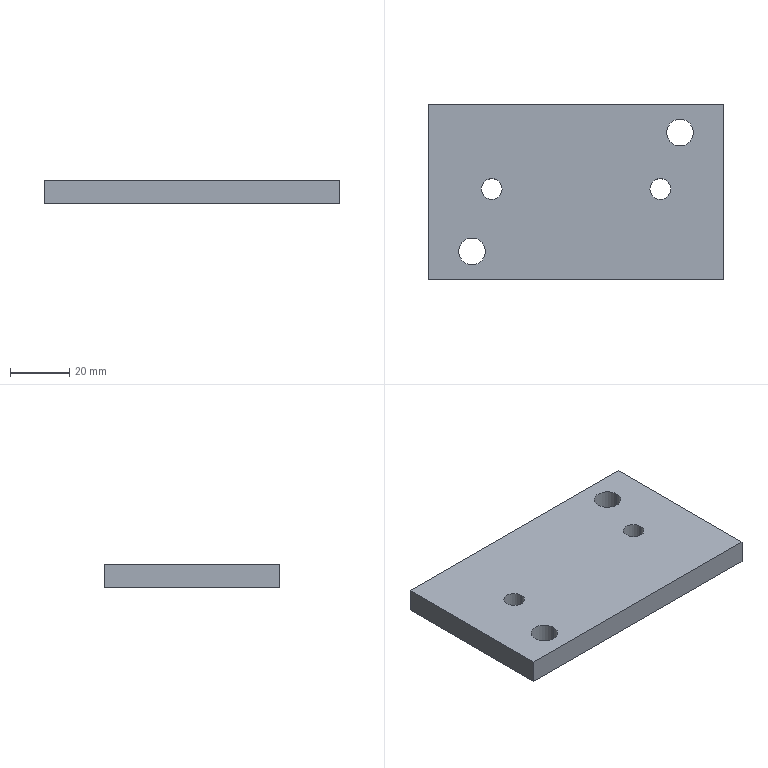Part | 1 solid | 14 faces | box 99 x 59 x 8 mm | volume 45095 mm3 | cylinder 8 | plane 6 | commonest cylinder face diameters 7 x4 9 x4
STEP:
#1=CARTESIAN_POINT('',(0.,0.,0.));
#2=DIRECTION('',(0.,0.,1.));
#3=DIRECTION('',(1.,0.,0.));
#4=AXIS2_PLACEMENT_3D('',#1,#2,#3);
#5=CARTESIAN_POINT('',(-190.5,445.,-105.051));
#6=VERTEX_POINT('',#5);
#7=CARTESIAN_POINT('',(-190.5,504.,-105.051));
#8=VERTEX_POINT('',#7);
#9=CARTESIAN_POINT('',(-190.5,445.,-105.051));
#10=DIRECTION('',(0.,1.,0.));
#11=VECTOR('',#10,1.);
#12=LINE('',#9,#11);
#13=CARTESIAN_POINT('',(-190.5,445.,-113.051));
#14=DIRECTION('',(1.,0.,0.));
#15=DIRECTION('',(0.,0.,1.));
#16=AXIS2_PLACEMENT_3D('',#13,#14,#15);
#17=PLANE('',#16);
#18=CARTESIAN_POINT('',(8.,0.));
#19=DIRECTION('',(0.,-1.));
#20=VECTOR('',#19,1.);
#21=LINE('',#18,#20);
#22=(GEOMETRIC_REPRESENTATION_CONTEXT(2)PARAMETRIC_REPRESENTATION_CONTEXT()REPRESENTATION_CONTEXT('',''));
#23=DEFINITIONAL_REPRESENTATION('',(#21),#22);
#24=PCURVE('',#17,#23);
#25=CARTESIAN_POINT('',(-211.613,475.5,-105.051));
#26=DIRECTION('',(0.,0.,1.));
#27=DIRECTION('',(-1.,0.,0.));
#28=AXIS2_PLACEMENT_3D('',#25,#26,#27);
#29=PLANE('',#28);
#30=CARTESIAN_POINT('',(-21.113,30.5));
#31=DIRECTION('',(0.,-1.));
#32=VECTOR('',#31,1.);
#33=LINE('',#30,#32);
#34=(GEOMETRIC_REPRESENTATION_CONTEXT(2)PARAMETRIC_REPRESENTATION_CONTEXT()REPRESENTATION_CONTEXT('',''));
#35=DEFINITIONAL_REPRESENTATION('',(#33),#34);
#36=PCURVE('',#29,#35);
#37=SURFACE_CURVE('',#12,(#24,#36),.PCURVE_S1.);
#38=EDGE_CURVE('',#6,#8,#37,.T.);
#39=ORIENTED_EDGE('',*,*,#38,.F.);
#40=CARTESIAN_POINT('',(-190.5,445.,-113.051));
#41=VERTEX_POINT('',#40);
#42=CARTESIAN_POINT('',(-190.5,445.,-113.051));
#43=DIRECTION('',(0.,0.,1.));
#44=VECTOR('',#43,1.);
#45=LINE('',#42,#44);
#46=CARTESIAN_POINT('',(0.,0.));
#47=DIRECTION('',(1.,0.));
#48=VECTOR('',#47,1.);
#49=LINE('',#46,#48);
#50=(GEOMETRIC_REPRESENTATION_CONTEXT(2)PARAMETRIC_REPRESENTATION_CONTEXT()REPRESENTATION_CONTEXT('',''));
#51=DEFINITIONAL_REPRESENTATION('',(#49),#50);
#52=PCURVE('',#17,#51);
#53=CARTESIAN_POINT('',(-289.5,445.,-113.051));
#54=DIRECTION('',(0.,-1.,0.));
#55=DIRECTION('',(0.,0.,1.));
#56=AXIS2_PLACEMENT_3D('',#53,#54,#55);
#57=PLANE('',#56);
#58=CARTESIAN_POINT('',(0.,-99.));
#59=DIRECTION('',(1.,0.));
#60=VECTOR('',#59,1.);
#61=LINE('',#58,#60);
#62=(GEOMETRIC_REPRESENTATION_CONTEXT(2)PARAMETRIC_REPRESENTATION_CONTEXT()REPRESENTATION_CONTEXT('',''));
#63=DEFINITIONAL_REPRESENTATION('',(#61),#62);
#64=PCURVE('',#57,#63);
#65=SURFACE_CURVE('',#45,(#52,#64),.PCURVE_S1.);
#66=EDGE_CURVE('',#41,#6,#65,.T.);
#67=ORIENTED_EDGE('',*,*,#66,.F.);
#68=CARTESIAN_POINT('',(-190.5,504.,-113.051));
#69=VERTEX_POINT('',#68);
#70=CARTESIAN_POINT('',(-190.5,445.,-113.051));
#71=DIRECTION('',(0.,1.,0.));
#72=VECTOR('',#71,1.);
#73=LINE('',#70,#72);
#74=CARTESIAN_POINT('',(0.,0.));
#75=DIRECTION('',(0.,-1.));
#76=VECTOR('',#75,1.);
#77=LINE('',#74,#76);
#78=(GEOMETRIC_REPRESENTATION_CONTEXT(2)PARAMETRIC_REPRESENTATION_CONTEXT()REPRESENTATION_CONTEXT('',''));
#79=DEFINITIONAL_REPRESENTATION('',(#77),#78);
#80=PCURVE('',#17,#79);
#81=CARTESIAN_POINT('',(-211.613,475.5,-113.051));
#82=DIRECTION('',(0.,0.,1.));
#83=DIRECTION('',(-1.,0.,0.));
#84=AXIS2_PLACEMENT_3D('',#81,#82,#83);
#85=PLANE('',#84);
#86=CARTESIAN_POINT('',(-21.113,30.5));
#87=DIRECTION('',(0.,-1.));
#88=VECTOR('',#87,1.);
#89=LINE('',#86,#88);
#90=(GEOMETRIC_REPRESENTATION_CONTEXT(2)PARAMETRIC_REPRESENTATION_CONTEXT()REPRESENTATION_CONTEXT('',''));
#91=DEFINITIONAL_REPRESENTATION('',(#89),#90);
#92=PCURVE('',#85,#91);
#93=SURFACE_CURVE('',#73,(#80,#92),.PCURVE_S1.);
#94=EDGE_CURVE('',#41,#69,#93,.T.);
#95=ORIENTED_EDGE('',*,*,#94,.T.);
#96=CARTESIAN_POINT('',(-190.5,504.,-113.051));
#97=DIRECTION('',(0.,0.,1.));
#98=VECTOR('',#97,1.);
#99=LINE('',#96,#98);
#100=CARTESIAN_POINT('',(0.,-59.));
#101=DIRECTION('',(1.,0.));
#102=VECTOR('',#101,1.);
#103=LINE('',#100,#102);
#104=(GEOMETRIC_REPRESENTATION_CONTEXT(2)PARAMETRIC_REPRESENTATION_CONTEXT()REPRESENTATION_CONTEXT('',''));
#105=DEFINITIONAL_REPRESENTATION('',(#103),#104);
#106=PCURVE('',#17,#105);
#107=CARTESIAN_POINT('',(-190.5,504.,-113.051));
#108=DIRECTION('',(0.,1.,0.));
#109=DIRECTION('',(0.,0.,-1.));
#110=AXIS2_PLACEMENT_3D('',#107,#108,#109);
#111=PLANE('',#110);
#112=CARTESIAN_POINT('',(0.,0.));
#113=DIRECTION('',(-1.,0.));
#114=VECTOR('',#113,1.);
#115=LINE('',#112,#114);
#116=(GEOMETRIC_REPRESENTATION_CONTEXT(2)PARAMETRIC_REPRESENTATION_CONTEXT()REPRESENTATION_CONTEXT('',''));
#117=DEFINITIONAL_REPRESENTATION('',(#115),#116);
#118=PCURVE('',#111,#117);
#119=SURFACE_CURVE('',#99,(#106,#118),.PCURVE_S1.);
#120=EDGE_CURVE('',#69,#8,#119,.T.);
#121=ORIENTED_EDGE('',*,*,#120,.T.);
#122=EDGE_LOOP('',(#39,#67,#95,#121));
#123=FACE_BOUND('',#122,.T.);
#124=ADVANCED_FACE('',(#123),#17,.T.);
#125=CARTESIAN_POINT('',(-289.5,504.,-105.051));
#126=VERTEX_POINT('',#125);
#127=CARTESIAN_POINT('',(-190.5,504.,-105.051));
#128=DIRECTION('',(-1.,0.,0.));
#129=VECTOR('',#128,1.);
#130=LINE('',#127,#129);
#131=CARTESIAN_POINT('',(-8.,0.));
#132=DIRECTION('',(0.,1.));
#133=VECTOR('',#132,1.);
#134=LINE('',#131,#133);
#135=(GEOMETRIC_REPRESENTATION_CONTEXT(2)PARAMETRIC_REPRESENTATION_CONTEXT()REPRESENTATION_CONTEXT('',''));
#136=DEFINITIONAL_REPRESENTATION('',(#134),#135);
#137=PCURVE('',#111,#136);
#138=CARTESIAN_POINT('',(-21.113,-28.5));
#139=DIRECTION('',(1.,0.));
#140=VECTOR('',#139,1.);
#141=LINE('',#138,#140);
#142=(GEOMETRIC_REPRESENTATION_CONTEXT(2)PARAMETRIC_REPRESENTATION_CONTEXT()REPRESENTATION_CONTEXT('',''));
#143=DEFINITIONAL_REPRESENTATION('',(#141),#142);
#144=PCURVE('',#29,#143);
#145=SURFACE_CURVE('',#130,(#137,#144),.PCURVE_S1.);
#146=EDGE_CURVE('',#8,#126,#145,.T.);
#147=ORIENTED_EDGE('',*,*,#146,.F.);
#148=ORIENTED_EDGE('',*,*,#120,.F.);
#149=CARTESIAN_POINT('',(-289.5,504.,-113.051));
#150=VERTEX_POINT('',#149);
#151=CARTESIAN_POINT('',(-190.5,504.,-113.051));
#152=DIRECTION('',(-1.,0.,0.));
#153=VECTOR('',#152,1.);
#154=LINE('',#151,#153);
#155=CARTESIAN_POINT('',(0.,0.));
#156=DIRECTION('',(0.,1.));
#157=VECTOR('',#156,1.);
#158=LINE('',#155,#157);
#159=(GEOMETRIC_REPRESENTATION_CONTEXT(2)PARAMETRIC_REPRESENTATION_CONTEXT()REPRESENTATION_CONTEXT('',''));
#160=DEFINITIONAL_REPRESENTATION('',(#158),#159);
#161=PCURVE('',#111,#160);
#162=CARTESIAN_POINT('',(-21.113,-28.5));
#163=DIRECTION('',(1.,0.));
#164=VECTOR('',#163,1.);
#165=LINE('',#162,#164);
#166=(GEOMETRIC_REPRESENTATION_CONTEXT(2)PARAMETRIC_REPRESENTATION_CONTEXT()REPRESENTATION_CONTEXT('',''));
#167=DEFINITIONAL_REPRESENTATION('',(#165),#166);
#168=PCURVE('',#85,#167);
#169=SURFACE_CURVE('',#154,(#161,#168),.PCURVE_S1.);
#170=EDGE_CURVE('',#69,#150,#169,.T.);
#171=ORIENTED_EDGE('',*,*,#170,.T.);
#172=CARTESIAN_POINT('',(-289.5,504.,-113.051));
#173=DIRECTION('',(0.,0.,1.));
#174=VECTOR('',#173,1.);
#175=LINE('',#172,#174);
#176=CARTESIAN_POINT('',(0.,99.));
#177=DIRECTION('',(-1.,0.));
#178=VECTOR('',#177,1.);
#179=LINE('',#176,#178);
#180=(GEOMETRIC_REPRESENTATION_CONTEXT(2)PARAMETRIC_REPRESENTATION_CONTEXT()REPRESENTATION_CONTEXT('',''));
#181=DEFINITIONAL_REPRESENTATION('',(#179),#180);
#182=PCURVE('',#111,#181);
#183=CARTESIAN_POINT('',(-289.5,504.,-113.051));
#184=DIRECTION('',(-1.,0.,0.));
#185=DIRECTION('',(0.,0.,-1.));
#186=AXIS2_PLACEMENT_3D('',#183,#184,#185);
#187=PLANE('',#186);
#188=CARTESIAN_POINT('',(0.,0.));
#189=DIRECTION('',(-1.,0.));
#190=VECTOR('',#189,1.);
#191=LINE('',#188,#190);
#192=(GEOMETRIC_REPRESENTATION_CONTEXT(2)PARAMETRIC_REPRESENTATION_CONTEXT()REPRESENTATION_CONTEXT('',''));
#193=DEFINITIONAL_REPRESENTATION('',(#191),#192);
#194=PCURVE('',#187,#193);
#195=SURFACE_CURVE('',#175,(#182,#194),.PCURVE_S1.);
#196=EDGE_CURVE('',#150,#126,#195,.T.);
#197=ORIENTED_EDGE('',*,*,#196,.T.);
#198=EDGE_LOOP('',(#147,#148,#171,#197));
#199=FACE_BOUND('',#198,.T.);
#200=ADVANCED_FACE('',(#199),#111,.T.);
#201=CARTESIAN_POINT('',(-289.5,445.,-105.051));
#202=VERTEX_POINT('',#201);
#203=CARTESIAN_POINT('',(-289.5,504.,-105.051));
#204=DIRECTION('',(0.,-1.,0.));
#205=VECTOR('',#204,1.);
#206=LINE('',#203,#205);
#207=CARTESIAN_POINT('',(-8.,0.));
#208=DIRECTION('',(0.,1.));
#209=VECTOR('',#208,1.);
#210=LINE('',#207,#209);
#211=(GEOMETRIC_REPRESENTATION_CONTEXT(2)PARAMETRIC_REPRESENTATION_CONTEXT()REPRESENTATION_CONTEXT('',''));
#212=DEFINITIONAL_REPRESENTATION('',(#210),#211);
#213=PCURVE('',#187,#212);
#214=CARTESIAN_POINT('',(77.887,-28.5));
#215=DIRECTION('',(0.,1.));
#216=VECTOR('',#215,1.);
#217=LINE('',#214,#216);
#218=(GEOMETRIC_REPRESENTATION_CONTEXT(2)PARAMETRIC_REPRESENTATION_CONTEXT()REPRESENTATION_CONTEXT('',''));
#219=DEFINITIONAL_REPRESENTATION('',(#217),#218);
#220=PCURVE('',#29,#219);
#221=SURFACE_CURVE('',#206,(#213,#220),.PCURVE_S1.);
#222=EDGE_CURVE('',#126,#202,#221,.T.);
#223=ORIENTED_EDGE('',*,*,#222,.F.);
#224=ORIENTED_EDGE('',*,*,#196,.F.);
#225=CARTESIAN_POINT('',(-289.5,445.,-113.051));
#226=VERTEX_POINT('',#225);
#227=CARTESIAN_POINT('',(-289.5,504.,-113.051));
#228=DIRECTION('',(0.,-1.,0.));
#229=VECTOR('',#228,1.);
#230=LINE('',#227,#229);
#231=CARTESIAN_POINT('',(0.,0.));
#232=DIRECTION('',(0.,1.));
#233=VECTOR('',#232,1.);
#234=LINE('',#231,#233);
#235=(GEOMETRIC_REPRESENTATION_CONTEXT(2)PARAMETRIC_REPRESENTATION_CONTEXT()REPRESENTATION_CONTEXT('',''));
#236=DEFINITIONAL_REPRESENTATION('',(#234),#235);
#237=PCURVE('',#187,#236);
#238=CARTESIAN_POINT('',(77.887,-28.5));
#239=DIRECTION('',(0.,1.));
#240=VECTOR('',#239,1.);
#241=LINE('',#238,#240);
#242=(GEOMETRIC_REPRESENTATION_CONTEXT(2)PARAMETRIC_REPRESENTATION_CONTEXT()REPRESENTATION_CONTEXT('',''));
#243=DEFINITIONAL_REPRESENTATION('',(#241),#242);
#244=PCURVE('',#85,#243);
#245=SURFACE_CURVE('',#230,(#237,#244),.PCURVE_S1.);
#246=EDGE_CURVE('',#150,#226,#245,.T.);
#247=ORIENTED_EDGE('',*,*,#246,.T.);
#248=CARTESIAN_POINT('',(-289.5,445.,-113.051));
#249=DIRECTION('',(0.,0.,1.));
#250=VECTOR('',#249,1.);
#251=LINE('',#248,#250);
#252=CARTESIAN_POINT('',(0.,59.));
#253=DIRECTION('',(-1.,0.));
#254=VECTOR('',#253,1.);
#255=LINE('',#252,#254);
#256=(GEOMETRIC_REPRESENTATION_CONTEXT(2)PARAMETRIC_REPRESENTATION_CONTEXT()REPRESENTATION_CONTEXT('',''));
#257=DEFINITIONAL_REPRESENTATION('',(#255),#256);
#258=PCURVE('',#187,#257);
#259=CARTESIAN_POINT('',(0.,0.));
#260=DIRECTION('',(1.,0.));
#261=VECTOR('',#260,1.);
#262=LINE('',#259,#261);
#263=(GEOMETRIC_REPRESENTATION_CONTEXT(2)PARAMETRIC_REPRESENTATION_CONTEXT()REPRESENTATION_CONTEXT('',''));
#264=DEFINITIONAL_REPRESENTATION('',(#262),#263);
#265=PCURVE('',#57,#264);
#266=SURFACE_CURVE('',#251,(#258,#265),.PCURVE_S1.);
#267=EDGE_CURVE('',#226,#202,#266,.T.);
#268=ORIENTED_EDGE('',*,*,#267,.T.);
#269=EDGE_LOOP('',(#223,#224,#247,#268));
#270=FACE_BOUND('',#269,.T.);
#271=ADVANCED_FACE('',(#270),#187,.T.);
#272=CARTESIAN_POINT('',(-289.5,445.,-105.051));
#273=DIRECTION('',(1.,0.,0.));
#274=VECTOR('',#273,1.);
#275=LINE('',#272,#274);
#276=CARTESIAN_POINT('',(8.,0.));
#277=DIRECTION('',(0.,-1.));
#278=VECTOR('',#277,1.);
#279=LINE('',#276,#278);
#280=(GEOMETRIC_REPRESENTATION_CONTEXT(2)PARAMETRIC_REPRESENTATION_CONTEXT()REPRESENTATION_CONTEXT('',''));
#281=DEFINITIONAL_REPRESENTATION('',(#279),#280);
#282=PCURVE('',#57,#281);
#283=CARTESIAN_POINT('',(77.887,30.5));
#284=DIRECTION('',(-1.,0.));
#285=VECTOR('',#284,1.);
#286=LINE('',#283,#285);
#287=(GEOMETRIC_REPRESENTATION_CONTEXT(2)PARAMETRIC_REPRESENTATION_CONTEXT()REPRESENTATION_CONTEXT('',''));
#288=DEFINITIONAL_REPRESENTATION('',(#286),#287);
#289=PCURVE('',#29,#288);
#290=SURFACE_CURVE('',#275,(#282,#289),.PCURVE_S1.);
#291=EDGE_CURVE('',#202,#6,#290,.T.);
#292=ORIENTED_EDGE('',*,*,#291,.F.);
#293=ORIENTED_EDGE('',*,*,#267,.F.);
#294=CARTESIAN_POINT('',(-289.5,445.,-113.051));
#295=DIRECTION('',(1.,0.,0.));
#296=VECTOR('',#295,1.);
#297=LINE('',#294,#296);
#298=CARTESIAN_POINT('',(0.,0.));
#299=DIRECTION('',(0.,-1.));
#300=VECTOR('',#299,1.);
#301=LINE('',#298,#300);
#302=(GEOMETRIC_REPRESENTATION_CONTEXT(2)PARAMETRIC_REPRESENTATION_CONTEXT()REPRESENTATION_CONTEXT('',''));
#303=DEFINITIONAL_REPRESENTATION('',(#301),#302);
#304=PCURVE('',#57,#303);
#305=CARTESIAN_POINT('',(77.887,30.5));
#306=DIRECTION('',(-1.,0.));
#307=VECTOR('',#306,1.);
#308=LINE('',#305,#307);
#309=(GEOMETRIC_REPRESENTATION_CONTEXT(2)PARAMETRIC_REPRESENTATION_CONTEXT()REPRESENTATION_CONTEXT('',''));
#310=DEFINITIONAL_REPRESENTATION('',(#308),#309);
#311=PCURVE('',#85,#310);
#312=SURFACE_CURVE('',#297,(#304,#311),.PCURVE_S1.);
#313=EDGE_CURVE('',#226,#41,#312,.T.);
#314=ORIENTED_EDGE('',*,*,#313,.T.);
#315=ORIENTED_EDGE('',*,*,#66,.T.);
#316=EDGE_LOOP('',(#292,#293,#314,#315));
#317=FACE_BOUND('',#316,.T.);
#318=ADVANCED_FACE('',(#317),#57,.T.);
#319=ORIENTED_EDGE('',*,*,#94,.F.);
#320=ORIENTED_EDGE('',*,*,#313,.F.);
#321=ORIENTED_EDGE('',*,*,#246,.F.);
#322=ORIENTED_EDGE('',*,*,#170,.F.);
#323=EDGE_LOOP('',(#319,#320,#321,#322));
#324=FACE_BOUND('',#323,.T.);
#325=CARTESIAN_POINT('',(-215.113,475.5,-113.051));
#326=VERTEX_POINT('',#325);
#327=CARTESIAN_POINT('',(-208.113,475.5,-113.051));
#328=VERTEX_POINT('',#327);
#329=CARTESIAN_POINT('',(-211.613,475.5,-113.051));
#330=DIRECTION('',(0.,0.,1.));
#331=DIRECTION('',(-1.,0.,0.));
#332=AXIS2_PLACEMENT_3D('',#329,#330,#331);
#333=CIRCLE('',#332,3.5);
#334=CARTESIAN_POINT('',(0.,0.));
#335=DIRECTION('',(1.,0.));
#336=AXIS2_PLACEMENT_2D('',#334,#335);
#337=CIRCLE('',#336,3.5);
#338=(GEOMETRIC_REPRESENTATION_CONTEXT(2)PARAMETRIC_REPRESENTATION_CONTEXT()REPRESENTATION_CONTEXT('',''));
#339=DEFINITIONAL_REPRESENTATION('',(#337),#338);
#340=PCURVE('',#85,#339);
#341=CARTESIAN_POINT('',(-211.613,475.5,-113.051));
#342=DIRECTION('',(0.,0.,1.));
#343=DIRECTION('',(0.,1.,0.));
#344=AXIS2_PLACEMENT_3D('',#341,#342,#343);
#345=CYLINDRICAL_SURFACE('',#344,3.5);
#346=CARTESIAN_POINT('',(1.571,0.));
#347=DIRECTION('',(1.,0.));
#348=VECTOR('',#347,1.);
#349=LINE('',#346,#348);
#350=(GEOMETRIC_REPRESENTATION_CONTEXT(2)PARAMETRIC_REPRESENTATION_CONTEXT()REPRESENTATION_CONTEXT('',''));
#351=DEFINITIONAL_REPRESENTATION('',(#349),#350);
#352=PCURVE('',#345,#351);
#353=SURFACE_CURVE('',#333,(#340,#352),.PCURVE_S1.);
#354=EDGE_CURVE('',#326,#328,#353,.T.);
#355=ORIENTED_EDGE('',*,*,#354,.T.);
#356=CARTESIAN_POINT('',(-211.613,475.5,-113.051));
#357=DIRECTION('',(0.,0.,1.));
#358=DIRECTION('',(-1.,0.,0.));
#359=AXIS2_PLACEMENT_3D('',#356,#357,#358);
#360=CIRCLE('',#359,3.5);
#361=CARTESIAN_POINT('',(0.,0.));
#362=DIRECTION('',(1.,0.));
#363=AXIS2_PLACEMENT_2D('',#361,#362);
#364=CIRCLE('',#363,3.5);
#365=(GEOMETRIC_REPRESENTATION_CONTEXT(2)PARAMETRIC_REPRESENTATION_CONTEXT()REPRESENTATION_CONTEXT('',''));
#366=DEFINITIONAL_REPRESENTATION('',(#364),#365);
#367=PCURVE('',#85,#366);
#368=CARTESIAN_POINT('',(-211.613,475.5,-113.051));
#369=DIRECTION('',(0.,0.,1.));
#370=DIRECTION('',(0.,-1.,0.));
#371=AXIS2_PLACEMENT_3D('',#368,#369,#370);
#372=CYLINDRICAL_SURFACE('',#371,3.5);
#373=CARTESIAN_POINT('',(-1.571,0.));
#374=DIRECTION('',(1.,0.));
#375=VECTOR('',#374,1.);
#376=LINE('',#373,#375);
#377=(GEOMETRIC_REPRESENTATION_CONTEXT(2)PARAMETRIC_REPRESENTATION_CONTEXT()REPRESENTATION_CONTEXT('',''));
#378=DEFINITIONAL_REPRESENTATION('',(#376),#377);
#379=PCURVE('',#372,#378);
#380=SURFACE_CURVE('',#360,(#367,#379),.PCURVE_S1.);
#381=EDGE_CURVE('',#328,#326,#380,.T.);
#382=ORIENTED_EDGE('',*,*,#381,.T.);
#383=EDGE_LOOP('',(#355,#382));
#384=FACE_BOUND('',#383,.T.);
#385=CARTESIAN_POINT('',(-209.5,494.5,-113.051));
#386=VERTEX_POINT('',#385);
#387=CARTESIAN_POINT('',(-200.5,494.5,-113.051));
#388=VERTEX_POINT('',#387);
#389=CARTESIAN_POINT('',(-205.,494.5,-113.051));
#390=DIRECTION('',(0.,0.,1.));
#391=DIRECTION('',(-1.,0.,0.));
#392=AXIS2_PLACEMENT_3D('',#389,#390,#391);
#393=CIRCLE('',#392,4.5);
#394=CARTESIAN_POINT('',(-6.613,-19.));
#395=DIRECTION('',(1.,0.));
#396=AXIS2_PLACEMENT_2D('',#394,#395);
#397=CIRCLE('',#396,4.5);
#398=(GEOMETRIC_REPRESENTATION_CONTEXT(2)PARAMETRIC_REPRESENTATION_CONTEXT()REPRESENTATION_CONTEXT('',''));
#399=DEFINITIONAL_REPRESENTATION('',(#397),#398);
#400=PCURVE('',#85,#399);
#401=CARTESIAN_POINT('',(-205.,494.5,-113.051));
#402=DIRECTION('',(0.,0.,1.));
#403=DIRECTION('',(0.,1.,0.));
#404=AXIS2_PLACEMENT_3D('',#401,#402,#403);
#405=CYLINDRICAL_SURFACE('',#404,4.5);
#406=CARTESIAN_POINT('',(1.571,0.));
#407=DIRECTION('',(1.,0.));
#408=VECTOR('',#407,1.);
#409=LINE('',#406,#408);
#410=(GEOMETRIC_REPRESENTATION_CONTEXT(2)PARAMETRIC_REPRESENTATION_CONTEXT()REPRESENTATION_CONTEXT('',''));
#411=DEFINITIONAL_REPRESENTATION('',(#409),#410);
#412=PCURVE('',#405,#411);
#413=SURFACE_CURVE('',#393,(#400,#412),.PCURVE_S1.);
#414=EDGE_CURVE('',#386,#388,#413,.T.);
#415=ORIENTED_EDGE('',*,*,#414,.T.);
#416=CARTESIAN_POINT('',(-205.,494.5,-113.051));
#417=DIRECTION('',(0.,0.,1.));
#418=DIRECTION('',(-1.,0.,0.));
#419=AXIS2_PLACEMENT_3D('',#416,#417,#418);
#420=CIRCLE('',#419,4.5);
#421=CARTESIAN_POINT('',(-6.613,-19.));
#422=DIRECTION('',(1.,0.));
#423=AXIS2_PLACEMENT_2D('',#421,#422);
#424=CIRCLE('',#423,4.5);
#425=(GEOMETRIC_REPRESENTATION_CONTEXT(2)PARAMETRIC_REPRESENTATION_CONTEXT()REPRESENTATION_CONTEXT('',''));
#426=DEFINITIONAL_REPRESENTATION('',(#424),#425);
#427=PCURVE('',#85,#426);
#428=CARTESIAN_POINT('',(-205.,494.5,-113.051));
#429=DIRECTION('',(0.,0.,1.));
#430=DIRECTION('',(0.,-1.,0.));
#431=AXIS2_PLACEMENT_3D('',#428,#429,#430);
#432=CYLINDRICAL_SURFACE('',#431,4.5);
#433=CARTESIAN_POINT('',(-1.571,0.));
#434=DIRECTION('',(1.,0.));
#435=VECTOR('',#434,1.);
#436=LINE('',#433,#435);
#437=(GEOMETRIC_REPRESENTATION_CONTEXT(2)PARAMETRIC_REPRESENTATION_CONTEXT()REPRESENTATION_CONTEXT('',''));
#438=DEFINITIONAL_REPRESENTATION('',(#436),#437);
#439=PCURVE('',#432,#438);
#440=SURFACE_CURVE('',#420,(#427,#439),.PCURVE_S1.);
#441=EDGE_CURVE('',#388,#386,#440,.T.);
#442=ORIENTED_EDGE('',*,*,#441,.T.);
#443=EDGE_LOOP('',(#415,#442));
#444=FACE_BOUND('',#443,.T.);
#445=CARTESIAN_POINT('',(-271.863,475.5,-113.051));
#446=VERTEX_POINT('',#445);
#447=CARTESIAN_POINT('',(-264.863,475.5,-113.051));
#448=VERTEX_POINT('',#447);
#449=CARTESIAN_POINT('',(-268.363,475.5,-113.051));
#450=DIRECTION('',(0.,0.,1.));
#451=DIRECTION('',(-1.,0.,0.));
#452=AXIS2_PLACEMENT_3D('',#449,#450,#451);
#453=CIRCLE('',#452,3.5);
#454=CARTESIAN_POINT('',(56.75,0.000000307));
#455=DIRECTION('',(1.,0.));
#456=AXIS2_PLACEMENT_2D('',#454,#455);
#457=CIRCLE('',#456,3.5);
#458=(GEOMETRIC_REPRESENTATION_CONTEXT(2)PARAMETRIC_REPRESENTATION_CONTEXT()REPRESENTATION_CONTEXT('',''));
#459=DEFINITIONAL_REPRESENTATION('',(#457),#458);
#460=PCURVE('',#85,#459);
#461=CARTESIAN_POINT('',(-268.363,475.5,-113.051));
#462=DIRECTION('',(0.,0.,1.));
#463=DIRECTION('',(0.,1.,0.));
#464=AXIS2_PLACEMENT_3D('',#461,#462,#463);
#465=CYLINDRICAL_SURFACE('',#464,3.5);
#466=CARTESIAN_POINT('',(1.571,0.));
#467=DIRECTION('',(1.,0.));
#468=VECTOR('',#467,1.);
#469=LINE('',#466,#468);
#470=(GEOMETRIC_REPRESENTATION_CONTEXT(2)PARAMETRIC_REPRESENTATION_CONTEXT()REPRESENTATION_CONTEXT('',''));
#471=DEFINITIONAL_REPRESENTATION('',(#469),#470);
#472=PCURVE('',#465,#471);
#473=SURFACE_CURVE('',#453,(#460,#472),.PCURVE_S1.);
#474=EDGE_CURVE('',#446,#448,#473,.T.);
#475=ORIENTED_EDGE('',*,*,#474,.T.);
#476=CARTESIAN_POINT('',(-268.363,475.5,-113.051));
#477=DIRECTION('',(0.,0.,1.));
#478=DIRECTION('',(-1.,0.,0.));
#479=AXIS2_PLACEMENT_3D('',#476,#477,#478);
#480=CIRCLE('',#479,3.5);
#481=CARTESIAN_POINT('',(56.75,0.000000307));
#482=DIRECTION('',(1.,0.));
#483=AXIS2_PLACEMENT_2D('',#481,#482);
#484=CIRCLE('',#483,3.5);
#485=(GEOMETRIC_REPRESENTATION_CONTEXT(2)PARAMETRIC_REPRESENTATION_CONTEXT()REPRESENTATION_CONTEXT('',''));
#486=DEFINITIONAL_REPRESENTATION('',(#484),#485);
#487=PCURVE('',#85,#486);
#488=CARTESIAN_POINT('',(-268.363,475.5,-113.051));
#489=DIRECTION('',(0.,0.,1.));
#490=DIRECTION('',(0.,-1.,0.));
#491=AXIS2_PLACEMENT_3D('',#488,#489,#490);
#492=CYLINDRICAL_SURFACE('',#491,3.5);
#493=CARTESIAN_POINT('',(-1.571,0.));
#494=DIRECTION('',(1.,0.));
#495=VECTOR('',#494,1.);
#496=LINE('',#493,#495);
#497=(GEOMETRIC_REPRESENTATION_CONTEXT(2)PARAMETRIC_REPRESENTATION_CONTEXT()REPRESENTATION_CONTEXT('',''));
#498=DEFINITIONAL_REPRESENTATION('',(#496),#497);
#499=PCURVE('',#492,#498);
#500=SURFACE_CURVE('',#480,(#487,#499),.PCURVE_S1.);
#501=EDGE_CURVE('',#448,#446,#500,.T.);
#502=ORIENTED_EDGE('',*,*,#501,.T.);
#503=EDGE_LOOP('',(#475,#502));
#504=FACE_BOUND('',#503,.T.);
#505=CARTESIAN_POINT('',(-279.5,454.5,-113.051));
#506=VERTEX_POINT('',#505);
#507=CARTESIAN_POINT('',(-270.5,454.5,-113.051));
#508=VERTEX_POINT('',#507);
#509=CARTESIAN_POINT('',(-275.,454.5,-113.051));
#510=DIRECTION('',(0.,0.,1.));
#511=DIRECTION('',(-1.,0.,0.));
#512=AXIS2_PLACEMENT_3D('',#509,#510,#511);
#513=CIRCLE('',#512,4.5);
#514=CARTESIAN_POINT('',(63.387,21.));
#515=DIRECTION('',(1.,0.));
#516=AXIS2_PLACEMENT_2D('',#514,#515);
#517=CIRCLE('',#516,4.5);
#518=(GEOMETRIC_REPRESENTATION_CONTEXT(2)PARAMETRIC_REPRESENTATION_CONTEXT()REPRESENTATION_CONTEXT('',''));
#519=DEFINITIONAL_REPRESENTATION('',(#517),#518);
#520=PCURVE('',#85,#519);
#521=CARTESIAN_POINT('',(-275.,454.5,-113.051));
#522=DIRECTION('',(0.,0.,1.));
#523=DIRECTION('',(0.,1.,0.));
#524=AXIS2_PLACEMENT_3D('',#521,#522,#523);
#525=CYLINDRICAL_SURFACE('',#524,4.5);
#526=CARTESIAN_POINT('',(1.571,0.));
#527=DIRECTION('',(1.,0.));
#528=VECTOR('',#527,1.);
#529=LINE('',#526,#528);
#530=(GEOMETRIC_REPRESENTATION_CONTEXT(2)PARAMETRIC_REPRESENTATION_CONTEXT()REPRESENTATION_CONTEXT('',''));
#531=DEFINITIONAL_REPRESENTATION('',(#529),#530);
#532=PCURVE('',#525,#531);
#533=SURFACE_CURVE('',#513,(#520,#532),.PCURVE_S1.);
#534=EDGE_CURVE('',#506,#508,#533,.T.);
#535=ORIENTED_EDGE('',*,*,#534,.T.);
#536=CARTESIAN_POINT('',(-275.,454.5,-113.051));
#537=DIRECTION('',(0.,0.,1.));
#538=DIRECTION('',(-1.,0.,0.));
#539=AXIS2_PLACEMENT_3D('',#536,#537,#538);
#540=CIRCLE('',#539,4.5);
#541=CARTESIAN_POINT('',(63.387,21.));
#542=DIRECTION('',(1.,0.));
#543=AXIS2_PLACEMENT_2D('',#541,#542);
#544=CIRCLE('',#543,4.5);
#545=(GEOMETRIC_REPRESENTATION_CONTEXT(2)PARAMETRIC_REPRESENTATION_CONTEXT()REPRESENTATION_CONTEXT('',''));
#546=DEFINITIONAL_REPRESENTATION('',(#544),#545);
#547=PCURVE('',#85,#546);
#548=CARTESIAN_POINT('',(-275.,454.5,-113.051));
#549=DIRECTION('',(0.,0.,1.));
#550=DIRECTION('',(0.,-1.,0.));
#551=AXIS2_PLACEMENT_3D('',#548,#549,#550);
#552=CYLINDRICAL_SURFACE('',#551,4.5);
#553=CARTESIAN_POINT('',(-1.571,0.));
#554=DIRECTION('',(1.,0.));
#555=VECTOR('',#554,1.);
#556=LINE('',#553,#555);
#557=(GEOMETRIC_REPRESENTATION_CONTEXT(2)PARAMETRIC_REPRESENTATION_CONTEXT()REPRESENTATION_CONTEXT('',''));
#558=DEFINITIONAL_REPRESENTATION('',(#556),#557);
#559=PCURVE('',#552,#558);
#560=SURFACE_CURVE('',#540,(#547,#559),.PCURVE_S1.);
#561=EDGE_CURVE('',#508,#506,#560,.T.);
#562=ORIENTED_EDGE('',*,*,#561,.T.);
#563=EDGE_LOOP('',(#535,#562));
#564=FACE_BOUND('',#563,.T.);
#565=ADVANCED_FACE('',(#324,#384,#444,#504,#564),#85,.F.);
#566=ORIENTED_EDGE('',*,*,#561,.T.);
#567=CARTESIAN_POINT('',(-279.5,454.5,-105.051));
#568=VERTEX_POINT('',#567);
#569=CARTESIAN_POINT('',(-279.5,454.5,-113.051));
#570=DIRECTION('',(0.,0.,1.));
#571=VECTOR('',#570,1.);
#572=LINE('',#569,#571);
#573=CARTESIAN_POINT('',(4.712,0.));
#574=DIRECTION('',(0.,1.));
#575=VECTOR('',#574,1.);
#576=LINE('',#573,#575);
#577=(GEOMETRIC_REPRESENTATION_CONTEXT(2)PARAMETRIC_REPRESENTATION_CONTEXT()REPRESENTATION_CONTEXT('',''));
#578=DEFINITIONAL_REPRESENTATION('',(#576),#577);
#579=PCURVE('',#552,#578);
#580=CARTESIAN_POINT('',(1.571,0.));
#581=DIRECTION('',(0.,1.));
#582=VECTOR('',#581,1.);
#583=LINE('',#580,#582);
#584=(GEOMETRIC_REPRESENTATION_CONTEXT(2)PARAMETRIC_REPRESENTATION_CONTEXT()REPRESENTATION_CONTEXT('',''));
#585=DEFINITIONAL_REPRESENTATION('',(#583),#584);
#586=PCURVE('',#525,#585);
#587=SURFACE_CURVE('',#572,(#579,#586),.PCURVE_S1.);
#588=EDGE_CURVE('',#506,#568,#587,.T.);
#589=ORIENTED_EDGE('',*,*,#588,.T.);
#590=CARTESIAN_POINT('',(-270.5,454.5,-105.051));
#591=VERTEX_POINT('',#590);
#592=CARTESIAN_POINT('',(-275.,454.5,-105.051));
#593=DIRECTION('',(0.,0.,1.));
#594=DIRECTION('',(-1.,0.,0.));
#595=AXIS2_PLACEMENT_3D('',#592,#593,#594);
#596=CIRCLE('',#595,4.5);
#597=CARTESIAN_POINT('',(-1.571,8.));
#598=DIRECTION('',(1.,0.));
#599=VECTOR('',#598,1.);
#600=LINE('',#597,#599);
#601=(GEOMETRIC_REPRESENTATION_CONTEXT(2)PARAMETRIC_REPRESENTATION_CONTEXT()REPRESENTATION_CONTEXT('',''));
#602=DEFINITIONAL_REPRESENTATION('',(#600),#601);
#603=PCURVE('',#552,#602);
#604=CARTESIAN_POINT('',(63.387,21.));
#605=DIRECTION('',(1.,0.));
#606=AXIS2_PLACEMENT_2D('',#604,#605);
#607=CIRCLE('',#606,4.5);
#608=(GEOMETRIC_REPRESENTATION_CONTEXT(2)PARAMETRIC_REPRESENTATION_CONTEXT()REPRESENTATION_CONTEXT('',''));
#609=DEFINITIONAL_REPRESENTATION('',(#607),#608);
#610=PCURVE('',#29,#609);
#611=SURFACE_CURVE('',#596,(#603,#610),.PCURVE_S1.);
#612=EDGE_CURVE('',#591,#568,#611,.T.);
#613=ORIENTED_EDGE('',*,*,#612,.F.);
#614=CARTESIAN_POINT('',(-270.5,454.5,-113.051));
#615=DIRECTION('',(0.,0.,1.));
#616=VECTOR('',#615,1.);
#617=LINE('',#614,#616);
#618=CARTESIAN_POINT('',(1.571,0.));
#619=DIRECTION('',(0.,1.));
#620=VECTOR('',#619,1.);
#621=LINE('',#618,#620);
#622=(GEOMETRIC_REPRESENTATION_CONTEXT(2)PARAMETRIC_REPRESENTATION_CONTEXT()REPRESENTATION_CONTEXT('',''));
#623=DEFINITIONAL_REPRESENTATION('',(#621),#622);
#624=PCURVE('',#552,#623);
#625=CARTESIAN_POINT('',(4.712,0.));
#626=DIRECTION('',(0.,1.));
#627=VECTOR('',#626,1.);
#628=LINE('',#625,#627);
#629=(GEOMETRIC_REPRESENTATION_CONTEXT(2)PARAMETRIC_REPRESENTATION_CONTEXT()REPRESENTATION_CONTEXT('',''));
#630=DEFINITIONAL_REPRESENTATION('',(#628),#629);
#631=PCURVE('',#525,#630);
#632=SURFACE_CURVE('',#617,(#624,#631),.PCURVE_S1.);
#633=EDGE_CURVE('',#508,#591,#632,.T.);
#634=ORIENTED_EDGE('',*,*,#633,.F.);
#635=EDGE_LOOP('',(#566,#589,#613,#634));
#636=FACE_BOUND('',#635,.F.);
#637=ADVANCED_FACE('',(#636),#552,.F.);
#638=ORIENTED_EDGE('',*,*,#38,.T.);
#639=ORIENTED_EDGE('',*,*,#146,.T.);
#640=ORIENTED_EDGE('',*,*,#222,.T.);
#641=ORIENTED_EDGE('',*,*,#291,.T.);
#642=EDGE_LOOP('',(#638,#639,#640,#641));
#643=FACE_BOUND('',#642,.T.);
#644=CARTESIAN_POINT('',(-208.113,475.5,-105.051));
#645=VERTEX_POINT('',#644);
#646=CARTESIAN_POINT('',(-215.113,475.5,-105.051));
#647=VERTEX_POINT('',#646);
#648=CARTESIAN_POINT('',(-211.613,475.5,-105.051));
#649=DIRECTION('',(0.,0.,1.));
#650=DIRECTION('',(-1.,0.,0.));
#651=AXIS2_PLACEMENT_3D('',#648,#649,#650);
#652=CIRCLE('',#651,3.5);
#653=CARTESIAN_POINT('',(0.,0.));
#654=DIRECTION('',(1.,0.));
#655=AXIS2_PLACEMENT_2D('',#653,#654);
#656=CIRCLE('',#655,3.5);
#657=(GEOMETRIC_REPRESENTATION_CONTEXT(2)PARAMETRIC_REPRESENTATION_CONTEXT()REPRESENTATION_CONTEXT('',''));
#658=DEFINITIONAL_REPRESENTATION('',(#656),#657);
#659=PCURVE('',#29,#658);
#660=CARTESIAN_POINT('',(-1.571,8.));
#661=DIRECTION('',(1.,0.));
#662=VECTOR('',#661,1.);
#663=LINE('',#660,#662);
#664=(GEOMETRIC_REPRESENTATION_CONTEXT(2)PARAMETRIC_REPRESENTATION_CONTEXT()REPRESENTATION_CONTEXT('',''));
#665=DEFINITIONAL_REPRESENTATION('',(#663),#664);
#666=PCURVE('',#372,#665);
#667=SURFACE_CURVE('',#652,(#659,#666),.PCURVE_S1.);
#668=EDGE_CURVE('',#645,#647,#667,.T.);
#669=ORIENTED_EDGE('',*,*,#668,.F.);
#670=CARTESIAN_POINT('',(-211.613,475.5,-105.051));
#671=DIRECTION('',(0.,0.,1.));
#672=DIRECTION('',(-1.,0.,0.));
#673=AXIS2_PLACEMENT_3D('',#670,#671,#672);
#674=CIRCLE('',#673,3.5);
#675=CARTESIAN_POINT('',(0.,0.));
#676=DIRECTION('',(1.,0.));
#677=AXIS2_PLACEMENT_2D('',#675,#676);
#678=CIRCLE('',#677,3.5);
#679=(GEOMETRIC_REPRESENTATION_CONTEXT(2)PARAMETRIC_REPRESENTATION_CONTEXT()REPRESENTATION_CONTEXT('',''));
#680=DEFINITIONAL_REPRESENTATION('',(#678),#679);
#681=PCURVE('',#29,#680);
#682=CARTESIAN_POINT('',(1.571,8.));
#683=DIRECTION('',(1.,0.));
#684=VECTOR('',#683,1.);
#685=LINE('',#682,#684);
#686=(GEOMETRIC_REPRESENTATION_CONTEXT(2)PARAMETRIC_REPRESENTATION_CONTEXT()REPRESENTATION_CONTEXT('',''));
#687=DEFINITIONAL_REPRESENTATION('',(#685),#686);
#688=PCURVE('',#345,#687);
#689=SURFACE_CURVE('',#674,(#681,#688),.PCURVE_S1.);
#690=EDGE_CURVE('',#647,#645,#689,.T.);
#691=ORIENTED_EDGE('',*,*,#690,.F.);
#692=EDGE_LOOP('',(#669,#691));
#693=FACE_BOUND('',#692,.T.);
#694=CARTESIAN_POINT('',(-200.5,494.5,-105.051));
#695=VERTEX_POINT('',#694);
#696=CARTESIAN_POINT('',(-209.5,494.5,-105.051));
#697=VERTEX_POINT('',#696);
#698=CARTESIAN_POINT('',(-205.,494.5,-105.051));
#699=DIRECTION('',(0.,0.,1.));
#700=DIRECTION('',(-1.,0.,0.));
#701=AXIS2_PLACEMENT_3D('',#698,#699,#700);
#702=CIRCLE('',#701,4.5);
#703=CARTESIAN_POINT('',(-6.613,-19.));
#704=DIRECTION('',(1.,0.));
#705=AXIS2_PLACEMENT_2D('',#703,#704);
#706=CIRCLE('',#705,4.5);
#707=(GEOMETRIC_REPRESENTATION_CONTEXT(2)PARAMETRIC_REPRESENTATION_CONTEXT()REPRESENTATION_CONTEXT('',''));
#708=DEFINITIONAL_REPRESENTATION('',(#706),#707);
#709=PCURVE('',#29,#708);
#710=CARTESIAN_POINT('',(-1.571,8.));
#711=DIRECTION('',(1.,0.));
#712=VECTOR('',#711,1.);
#713=LINE('',#710,#712);
#714=(GEOMETRIC_REPRESENTATION_CONTEXT(2)PARAMETRIC_REPRESENTATION_CONTEXT()REPRESENTATION_CONTEXT('',''));
#715=DEFINITIONAL_REPRESENTATION('',(#713),#714);
#716=PCURVE('',#432,#715);
#717=SURFACE_CURVE('',#702,(#709,#716),.PCURVE_S1.);
#718=EDGE_CURVE('',#695,#697,#717,.T.);
#719=ORIENTED_EDGE('',*,*,#718,.F.);
#720=CARTESIAN_POINT('',(-205.,494.5,-105.051));
#721=DIRECTION('',(0.,0.,1.));
#722=DIRECTION('',(-1.,0.,0.));
#723=AXIS2_PLACEMENT_3D('',#720,#721,#722);
#724=CIRCLE('',#723,4.5);
#725=CARTESIAN_POINT('',(-6.613,-19.));
#726=DIRECTION('',(1.,0.));
#727=AXIS2_PLACEMENT_2D('',#725,#726);
#728=CIRCLE('',#727,4.5);
#729=(GEOMETRIC_REPRESENTATION_CONTEXT(2)PARAMETRIC_REPRESENTATION_CONTEXT()REPRESENTATION_CONTEXT('',''));
#730=DEFINITIONAL_REPRESENTATION('',(#728),#729);
#731=PCURVE('',#29,#730);
#732=CARTESIAN_POINT('',(1.571,8.));
#733=DIRECTION('',(1.,0.));
#734=VECTOR('',#733,1.);
#735=LINE('',#732,#734);
#736=(GEOMETRIC_REPRESENTATION_CONTEXT(2)PARAMETRIC_REPRESENTATION_CONTEXT()REPRESENTATION_CONTEXT('',''));
#737=DEFINITIONAL_REPRESENTATION('',(#735),#736);
#738=PCURVE('',#405,#737);
#739=SURFACE_CURVE('',#724,(#731,#738),.PCURVE_S1.);
#740=EDGE_CURVE('',#697,#695,#739,.T.);
#741=ORIENTED_EDGE('',*,*,#740,.F.);
#742=EDGE_LOOP('',(#719,#741));
#743=FACE_BOUND('',#742,.T.);
#744=CARTESIAN_POINT('',(-264.863,475.5,-105.051));
#745=VERTEX_POINT('',#744);
#746=CARTESIAN_POINT('',(-271.863,475.5,-105.051));
#747=VERTEX_POINT('',#746);
#748=CARTESIAN_POINT('',(-268.363,475.5,-105.051));
#749=DIRECTION('',(0.,0.,1.));
#750=DIRECTION('',(-1.,0.,0.));
#751=AXIS2_PLACEMENT_3D('',#748,#749,#750);
#752=CIRCLE('',#751,3.5);
#753=CARTESIAN_POINT('',(56.75,0.000000307));
#754=DIRECTION('',(1.,0.));
#755=AXIS2_PLACEMENT_2D('',#753,#754);
#756=CIRCLE('',#755,3.5);
#757=(GEOMETRIC_REPRESENTATION_CONTEXT(2)PARAMETRIC_REPRESENTATION_CONTEXT()REPRESENTATION_CONTEXT('',''));
#758=DEFINITIONAL_REPRESENTATION('',(#756),#757);
#759=PCURVE('',#29,#758);
#760=CARTESIAN_POINT('',(-1.571,8.));
#761=DIRECTION('',(1.,0.));
#762=VECTOR('',#761,1.);
#763=LINE('',#760,#762);
#764=(GEOMETRIC_REPRESENTATION_CONTEXT(2)PARAMETRIC_REPRESENTATION_CONTEXT()REPRESENTATION_CONTEXT('',''));
#765=DEFINITIONAL_REPRESENTATION('',(#763),#764);
#766=PCURVE('',#492,#765);
#767=SURFACE_CURVE('',#752,(#759,#766),.PCURVE_S1.);
#768=EDGE_CURVE('',#745,#747,#767,.T.);
#769=ORIENTED_EDGE('',*,*,#768,.F.);
#770=CARTESIAN_POINT('',(-268.363,475.5,-105.051));
#771=DIRECTION('',(0.,0.,1.));
#772=DIRECTION('',(-1.,0.,0.));
#773=AXIS2_PLACEMENT_3D('',#770,#771,#772);
#774=CIRCLE('',#773,3.5);
#775=CARTESIAN_POINT('',(56.75,0.000000307));
#776=DIRECTION('',(1.,0.));
#777=AXIS2_PLACEMENT_2D('',#775,#776);
#778=CIRCLE('',#777,3.5);
#779=(GEOMETRIC_REPRESENTATION_CONTEXT(2)PARAMETRIC_REPRESENTATION_CONTEXT()REPRESENTATION_CONTEXT('',''));
#780=DEFINITIONAL_REPRESENTATION('',(#778),#779);
#781=PCURVE('',#29,#780);
#782=CARTESIAN_POINT('',(1.571,8.));
#783=DIRECTION('',(1.,0.));
#784=VECTOR('',#783,1.);
#785=LINE('',#782,#784);
#786=(GEOMETRIC_REPRESENTATION_CONTEXT(2)PARAMETRIC_REPRESENTATION_CONTEXT()REPRESENTATION_CONTEXT('',''));
#787=DEFINITIONAL_REPRESENTATION('',(#785),#786);
#788=PCURVE('',#465,#787);
#789=SURFACE_CURVE('',#774,(#781,#788),.PCURVE_S1.);
#790=EDGE_CURVE('',#747,#745,#789,.T.);
#791=ORIENTED_EDGE('',*,*,#790,.F.);
#792=EDGE_LOOP('',(#769,#791));
#793=FACE_BOUND('',#792,.T.);
#794=ORIENTED_EDGE('',*,*,#612,.F.);
#795=CARTESIAN_POINT('',(-275.,454.5,-105.051));
#796=DIRECTION('',(0.,0.,1.));
#797=DIRECTION('',(-1.,0.,0.));
#798=AXIS2_PLACEMENT_3D('',#795,#796,#797);
#799=CIRCLE('',#798,4.5);
#800=CARTESIAN_POINT('',(63.387,21.));
#801=DIRECTION('',(1.,0.));
#802=AXIS2_PLACEMENT_2D('',#800,#801);
#803=CIRCLE('',#802,4.5);
#804=(GEOMETRIC_REPRESENTATION_CONTEXT(2)PARAMETRIC_REPRESENTATION_CONTEXT()REPRESENTATION_CONTEXT('',''));
#805=DEFINITIONAL_REPRESENTATION('',(#803),#804);
#806=PCURVE('',#29,#805);
#807=CARTESIAN_POINT('',(1.571,8.));
#808=DIRECTION('',(1.,0.));
#809=VECTOR('',#808,1.);
#810=LINE('',#807,#809);
#811=(GEOMETRIC_REPRESENTATION_CONTEXT(2)PARAMETRIC_REPRESENTATION_CONTEXT()REPRESENTATION_CONTEXT('',''));
#812=DEFINITIONAL_REPRESENTATION('',(#810),#811);
#813=PCURVE('',#525,#812);
#814=SURFACE_CURVE('',#799,(#806,#813),.PCURVE_S1.);
#815=EDGE_CURVE('',#568,#591,#814,.T.);
#816=ORIENTED_EDGE('',*,*,#815,.F.);
#817=EDGE_LOOP('',(#794,#816));
#818=FACE_BOUND('',#817,.T.);
#819=ADVANCED_FACE('',(#643,#693,#743,#793,#818),#29,.T.);
#820=ORIENTED_EDGE('',*,*,#501,.T.);
#821=CARTESIAN_POINT('',(-271.863,475.5,-113.051));
#822=DIRECTION('',(0.,0.,1.));
#823=VECTOR('',#822,1.);
#824=LINE('',#821,#823);
#825=CARTESIAN_POINT('',(4.712,0.));
#826=DIRECTION('',(0.,1.));
#827=VECTOR('',#826,1.);
#828=LINE('',#825,#827);
#829=(GEOMETRIC_REPRESENTATION_CONTEXT(2)PARAMETRIC_REPRESENTATION_CONTEXT()REPRESENTATION_CONTEXT('',''));
#830=DEFINITIONAL_REPRESENTATION('',(#828),#829);
#831=PCURVE('',#492,#830);
#832=CARTESIAN_POINT('',(1.571,0.));
#833=DIRECTION('',(0.,1.));
#834=VECTOR('',#833,1.);
#835=LINE('',#832,#834);
#836=(GEOMETRIC_REPRESENTATION_CONTEXT(2)PARAMETRIC_REPRESENTATION_CONTEXT()REPRESENTATION_CONTEXT('',''));
#837=DEFINITIONAL_REPRESENTATION('',(#835),#836);
#838=PCURVE('',#465,#837);
#839=SURFACE_CURVE('',#824,(#831,#838),.PCURVE_S1.);
#840=EDGE_CURVE('',#446,#747,#839,.T.);
#841=ORIENTED_EDGE('',*,*,#840,.T.);
#842=ORIENTED_EDGE('',*,*,#768,.F.);
#843=CARTESIAN_POINT('',(-264.863,475.5,-113.051));
#844=DIRECTION('',(0.,0.,1.));
#845=VECTOR('',#844,1.);
#846=LINE('',#843,#845);
#847=CARTESIAN_POINT('',(1.571,0.));
#848=DIRECTION('',(0.,1.));
#849=VECTOR('',#848,1.);
#850=LINE('',#847,#849);
#851=(GEOMETRIC_REPRESENTATION_CONTEXT(2)PARAMETRIC_REPRESENTATION_CONTEXT()REPRESENTATION_CONTEXT('',''));
#852=DEFINITIONAL_REPRESENTATION('',(#850),#851);
#853=PCURVE('',#492,#852);
#854=CARTESIAN_POINT('',(4.712,0.));
#855=DIRECTION('',(0.,1.));
#856=VECTOR('',#855,1.);
#857=LINE('',#854,#856);
#858=(GEOMETRIC_REPRESENTATION_CONTEXT(2)PARAMETRIC_REPRESENTATION_CONTEXT()REPRESENTATION_CONTEXT('',''));
#859=DEFINITIONAL_REPRESENTATION('',(#857),#858);
#860=PCURVE('',#465,#859);
#861=SURFACE_CURVE('',#846,(#853,#860),.PCURVE_S1.);
#862=EDGE_CURVE('',#448,#745,#861,.T.);
#863=ORIENTED_EDGE('',*,*,#862,.F.);
#864=EDGE_LOOP('',(#820,#841,#842,#863));
#865=FACE_BOUND('',#864,.F.);
#866=ADVANCED_FACE('',(#865),#492,.F.);
#867=ORIENTED_EDGE('',*,*,#441,.T.);
#868=CARTESIAN_POINT('',(-209.5,494.5,-113.051));
#869=DIRECTION('',(0.,0.,1.));
#870=VECTOR('',#869,1.);
#871=LINE('',#868,#870);
#872=CARTESIAN_POINT('',(4.712,0.));
#873=DIRECTION('',(0.,1.));
#874=VECTOR('',#873,1.);
#875=LINE('',#872,#874);
#876=(GEOMETRIC_REPRESENTATION_CONTEXT(2)PARAMETRIC_REPRESENTATION_CONTEXT()REPRESENTATION_CONTEXT('',''));
#877=DEFINITIONAL_REPRESENTATION('',(#875),#876);
#878=PCURVE('',#432,#877);
#879=CARTESIAN_POINT('',(1.571,0.));
#880=DIRECTION('',(0.,1.));
#881=VECTOR('',#880,1.);
#882=LINE('',#879,#881);
#883=(GEOMETRIC_REPRESENTATION_CONTEXT(2)PARAMETRIC_REPRESENTATION_CONTEXT()REPRESENTATION_CONTEXT('',''));
#884=DEFINITIONAL_REPRESENTATION('',(#882),#883);
#885=PCURVE('',#405,#884);
#886=SURFACE_CURVE('',#871,(#878,#885),.PCURVE_S1.);
#887=EDGE_CURVE('',#386,#697,#886,.T.);
#888=ORIENTED_EDGE('',*,*,#887,.T.);
#889=ORIENTED_EDGE('',*,*,#718,.F.);
#890=CARTESIAN_POINT('',(-200.5,494.5,-113.051));
#891=DIRECTION('',(0.,0.,1.));
#892=VECTOR('',#891,1.);
#893=LINE('',#890,#892);
#894=CARTESIAN_POINT('',(1.571,0.));
#895=DIRECTION('',(0.,1.));
#896=VECTOR('',#895,1.);
#897=LINE('',#894,#896);
#898=(GEOMETRIC_REPRESENTATION_CONTEXT(2)PARAMETRIC_REPRESENTATION_CONTEXT()REPRESENTATION_CONTEXT('',''));
#899=DEFINITIONAL_REPRESENTATION('',(#897),#898);
#900=PCURVE('',#432,#899);
#901=CARTESIAN_POINT('',(4.712,0.));
#902=DIRECTION('',(0.,1.));
#903=VECTOR('',#902,1.);
#904=LINE('',#901,#903);
#905=(GEOMETRIC_REPRESENTATION_CONTEXT(2)PARAMETRIC_REPRESENTATION_CONTEXT()REPRESENTATION_CONTEXT('',''));
#906=DEFINITIONAL_REPRESENTATION('',(#904),#905);
#907=PCURVE('',#405,#906);
#908=SURFACE_CURVE('',#893,(#900,#907),.PCURVE_S1.);
#909=EDGE_CURVE('',#388,#695,#908,.T.);
#910=ORIENTED_EDGE('',*,*,#909,.F.);
#911=EDGE_LOOP('',(#867,#888,#889,#910));
#912=FACE_BOUND('',#911,.F.);
#913=ADVANCED_FACE('',(#912),#432,.F.);
#914=ORIENTED_EDGE('',*,*,#381,.T.);
#915=CARTESIAN_POINT('',(-215.113,475.5,-113.051));
#916=DIRECTION('',(0.,0.,1.));
#917=VECTOR('',#916,1.);
#918=LINE('',#915,#917);
#919=CARTESIAN_POINT('',(4.712,0.));
#920=DIRECTION('',(0.,1.));
#921=VECTOR('',#920,1.);
#922=LINE('',#919,#921);
#923=(GEOMETRIC_REPRESENTATION_CONTEXT(2)PARAMETRIC_REPRESENTATION_CONTEXT()REPRESENTATION_CONTEXT('',''));
#924=DEFINITIONAL_REPRESENTATION('',(#922),#923);
#925=PCURVE('',#372,#924);
#926=CARTESIAN_POINT('',(1.571,0.));
#927=DIRECTION('',(0.,1.));
#928=VECTOR('',#927,1.);
#929=LINE('',#926,#928);
#930=(GEOMETRIC_REPRESENTATION_CONTEXT(2)PARAMETRIC_REPRESENTATION_CONTEXT()REPRESENTATION_CONTEXT('',''));
#931=DEFINITIONAL_REPRESENTATION('',(#929),#930);
#932=PCURVE('',#345,#931);
#933=SURFACE_CURVE('',#918,(#925,#932),.PCURVE_S1.);
#934=EDGE_CURVE('',#326,#647,#933,.T.);
#935=ORIENTED_EDGE('',*,*,#934,.T.);
#936=ORIENTED_EDGE('',*,*,#668,.F.);
#937=CARTESIAN_POINT('',(-208.113,475.5,-113.051));
#938=DIRECTION('',(0.,0.,1.));
#939=VECTOR('',#938,1.);
#940=LINE('',#937,#939);
#941=CARTESIAN_POINT('',(1.571,0.));
#942=DIRECTION('',(0.,1.));
#943=VECTOR('',#942,1.);
#944=LINE('',#941,#943);
#945=(GEOMETRIC_REPRESENTATION_CONTEXT(2)PARAMETRIC_REPRESENTATION_CONTEXT()REPRESENTATION_CONTEXT('',''));
#946=DEFINITIONAL_REPRESENTATION('',(#944),#945);
#947=PCURVE('',#372,#946);
#948=CARTESIAN_POINT('',(4.712,0.));
#949=DIRECTION('',(0.,1.));
#950=VECTOR('',#949,1.);
#951=LINE('',#948,#950);
#952=(GEOMETRIC_REPRESENTATION_CONTEXT(2)PARAMETRIC_REPRESENTATION_CONTEXT()REPRESENTATION_CONTEXT('',''));
#953=DEFINITIONAL_REPRESENTATION('',(#951),#952);
#954=PCURVE('',#345,#953);
#955=SURFACE_CURVE('',#940,(#947,#954),.PCURVE_S1.);
#956=EDGE_CURVE('',#328,#645,#955,.T.);
#957=ORIENTED_EDGE('',*,*,#956,.F.);
#958=EDGE_LOOP('',(#914,#935,#936,#957));
#959=FACE_BOUND('',#958,.F.);
#960=ADVANCED_FACE('',(#959),#372,.F.);
#961=ORIENTED_EDGE('',*,*,#815,.F.);
#962=ORIENTED_EDGE('',*,*,#588,.F.);
#963=ORIENTED_EDGE('',*,*,#534,.T.);
#964=ORIENTED_EDGE('',*,*,#633,.T.);
#965=EDGE_LOOP('',(#961,#962,#963,#964));
#966=FACE_BOUND('',#965,.F.);
#967=ADVANCED_FACE('',(#966),#525,.F.);
#968=ORIENTED_EDGE('',*,*,#790,.F.);
#969=ORIENTED_EDGE('',*,*,#840,.F.);
#970=ORIENTED_EDGE('',*,*,#474,.T.);
#971=ORIENTED_EDGE('',*,*,#862,.T.);
#972=EDGE_LOOP('',(#968,#969,#970,#971));
#973=FACE_BOUND('',#972,.F.);
#974=ADVANCED_FACE('',(#973),#465,.F.);
#975=ORIENTED_EDGE('',*,*,#740,.F.);
#976=ORIENTED_EDGE('',*,*,#887,.F.);
#977=ORIENTED_EDGE('',*,*,#414,.T.);
#978=ORIENTED_EDGE('',*,*,#909,.T.);
#979=EDGE_LOOP('',(#975,#976,#977,#978));
#980=FACE_BOUND('',#979,.F.);
#981=ADVANCED_FACE('',(#980),#405,.F.);
#982=ORIENTED_EDGE('',*,*,#690,.F.);
#983=ORIENTED_EDGE('',*,*,#934,.F.);
#984=ORIENTED_EDGE('',*,*,#354,.T.);
#985=ORIENTED_EDGE('',*,*,#956,.T.);
#986=EDGE_LOOP('',(#982,#983,#984,#985));
#987=FACE_BOUND('',#986,.F.);
#988=ADVANCED_FACE('',(#987),#345,.F.);
#989=CLOSED_SHELL('',(#124,#200,#271,#318,#565,#637,#819,#866,#913,#960,#967,#974,#981,#988));
#990=MANIFOLD_SOLID_BREP('',#989);
#991=(LENGTH_UNIT()NAMED_UNIT(*)SI_UNIT(.MILLI.,.METRE.));
#992=UNCERTAINTY_MEASURE_WITH_UNIT(LENGTH_MEASURE(0.0000001),#991,'','');
#993=(NAMED_UNIT(*)PLANE_ANGLE_UNIT()SI_UNIT($,.RADIAN.));
#994=(NAMED_UNIT(*)SI_UNIT($,.STERADIAN.)SOLID_ANGLE_UNIT());
#995=(GEOMETRIC_REPRESENTATION_CONTEXT(3)GLOBAL_UNCERTAINTY_ASSIGNED_CONTEXT((#992))GLOBAL_UNIT_ASSIGNED_CONTEXT((#991,#993,#994))REPRESENTATION_CONTEXT('',''));
#996=ADVANCED_BREP_SHAPE_REPRESENTATION('',(#4,#990),#995);